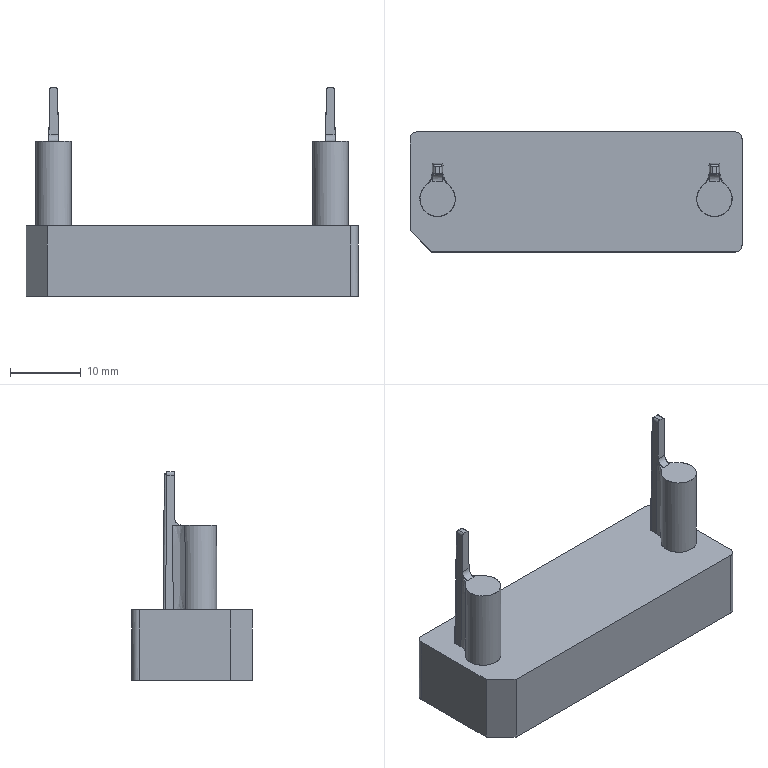CAM job | PowerMill | 3-axis milling, other | part box 47 x 17 x 29.578 mm
Tools:
number,name,type,diameter,tip_radius,length,cutting_length,overhang,flutes,holder,toolpaths_using
1,D10C_1_1_1,end_mill,10.0,0.0,60.0,,30.04,1,D42L35,6
3,D10_1_1_1,end_mill,10.0,0.0,60.0,,29.72,1,D42L35,6
14,D4_1_1,end_mill,4.0,0.0,30.0,,19.72,1,D42L35,1
13,Text_D4_1_1,taper_spherical,4.0,0.3,60.0,,19.84,1,D42L35,2
14,D4_2_1,end_mill,4.0,0.0,30.0,,19.6,1,D42L35,1
Operations:
program,toolpath,strategy,tool,tool_number,tool_diameter,tip_radius,flutes,spindle_rpm,feed_cut,surface_speed_m_min_computed,feed_per_tooth_computed,tolerance,thickness,stepover,stepdown,cut_length,cut_time_min,total_time_min,workplane
10-C01-8-F,精公开粗01-扫面平行-D10C,raster_area_clear,D10C_1_1_1,1,10.0,0.0,1.0,8000.0,10000.0,251.33,1.25,0.03,0.28,6.0,1.0,285.36,0.029,0.035,
10-C01-8-F,精公开粗01-外形偏置-D10C,offset_area_clear,D10C_1_1_1,1,10.0,0.0,1.0,8000.0,10000.0,251.33,1.25,0.03,0.28,6.0,1.0,16758.272,1.676,1.798,
10-C01-8-F,精公开粗01-基准台等高-D10C,constantz,D10C_1_1_1,1,10.0,0.0,1.0,8000.0,10000.0,251.33,1.25,0.03,0.07,5.0,0.4,4232.936,0.423,0.4354,
10-C01-8-F,精公基准台01-平坦面偏置-D10,offset_area_clear,D10_1_1_1,3,10.0,0.0,1.0,8500.0,600.0,267.04,0.0706,0.005,0.38,5.0,1.0,82.619,0.138,0.2033,
10-C01-8-F,精公基准台01-基准面偏置-D10,offset_area_clear,D10_1_1_1,3,10.0,0.0,1.0,8500.0,600.0,267.04,0.0706,0.005,0.38,5.0,1.0,233.686,0.39,0.4336,
10-C01-8-F,精公基准台01-基准台侧光-D10,profile_area_clear,D10_1_1_1,3,10.0,0.0,1.0,8500.0,600.0,267.04,0.0706,0.005,0.0,0.08,1.0,313.234,0.522,0.589,
10-C01-8-F,精公精光01-等高-D4,constantz,D4_1_1,14,4.0,0.0,1.0,18000.0,2000.0,226.19,0.1111,0.005,-0.075,5.0,0.02,26923.181,13.462,15.186,
10-C01-8-F,精公刻字01-刻字-Text_D4,pattern,Text_D4_1_1,13,4.0,0.3,1.0,15000.0,1000.0,188.5,0.0667,0.005,0.0,5.0,1.0,56.018,0.056,0.0765,
10-C01-8-R,粗公开粗01-扫面平行-D10C,raster_area_clear,D10C_1_1_1,1,10.0,0.0,1.0,8000.0,10000.0,251.33,1.25,0.03,0.15,6.0,1.0,567.6,0.057,0.0642,
10-C01-8-R,粗公开粗01-外形偏置-D10C,offset_area_clear,D10C_1_1_1,1,10.0,0.0,1.0,8000.0,10000.0,251.33,1.25,0.03,0.15,6.0,1.0,16619.755,1.662,1.785,
10-C01-8-R,粗公开粗01-基准台等高-D10C,constantz,D10C_1_1_1,1,10.0,0.0,1.0,8000.0,10000.0,251.33,1.25,0.03,0.07,5.0,0.4,4232.936,0.423,0.4354,
10-C01-8-R,粗公基准台01-平坦面偏置-D10,offset_area_clear,D10_1_1_1,3,10.0,0.0,1.0,8500.0,600.0,267.04,0.0706,0.01,0.25,5.0,1.0,79.315,0.132,0.1974,
10-C01-8-R,粗公基准台01-基准面偏置-D10,offset_area_clear,D10_1_1_1,3,10.0,0.0,1.0,8500.0,600.0,267.04,0.0706,0.01,0.25,5.0,1.0,231.752,0.386,0.4304,
10-C01-8-R,粗公基准台01-基准台侧光-D10,profile_area_clear,D10_1_1_1,3,10.0,0.0,1.0,8500.0,600.0,267.04,0.0706,0.01,0.0,0.08,1.0,313.217,0.522,0.5889,
10-C01-8-R,粗公精光01-等高-D4,constantz,D4_2_1,14,4.0,0.0,1.0,18000.0,2000.0,226.19,0.1111,0.01,-0.205,5.0,0.02,21916.631,10.958,12.427,
10-C01-8-R,粗公刻字01-刻字-Text_D4,pattern,Text_D4_1_1,13,4.0,0.3,1.0,15000.0,1000.0,188.5,0.0667,0.01,0.0,5.0,1.0,55.799,0.056,0.0755,